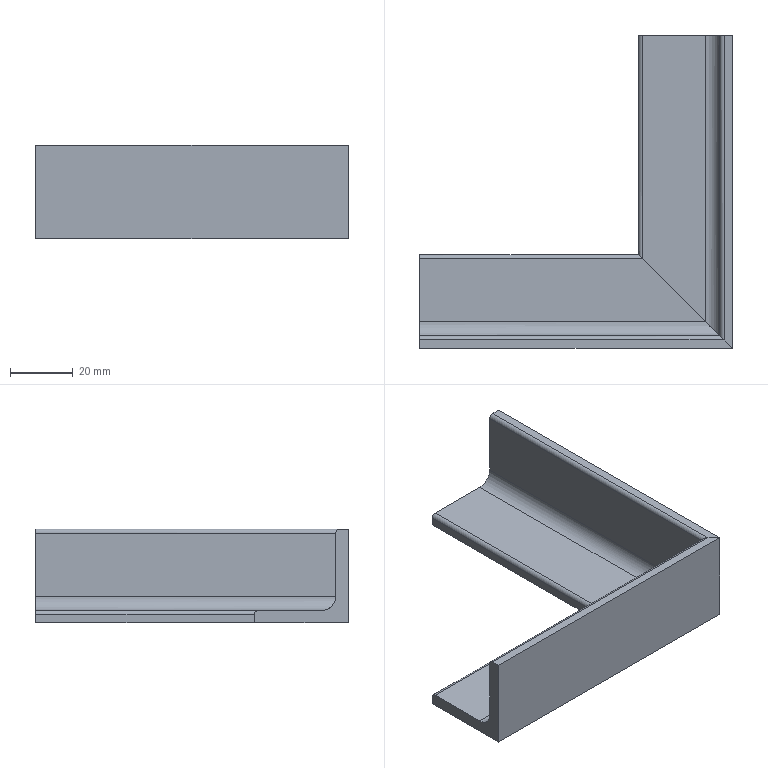Part | SolidWorks | features WeldMemberFeat 1, WeldmentFeature 1 | 2 solids | 22 faces | box 100 x 100 x 30 mm | volume 41483 mm3 | plane 16 | cylinder 6 | commonest cylinder face diameters 2.667 x4 9 x2
STEP:
#1=CARTESIAN_POINT('',(100.,0.,0.));
#2=VERTEX_POINT('',#1);
#3=CARTESIAN_POINT('',(70.,30.,0.));
#4=VERTEX_POINT('',#3);
#5=CARTESIAN_POINT('',(85.,15.,0.));
#6=DIRECTION('',(-0.7071,0.7071,0.));
#7=VECTOR('',#6,1000.);
#8=LINE('',#5,#7);
#9=EDGE_CURVE('',#2,#4,#8,.T.);
#10=ORIENTED_EDGE('',*,*,#9,.F.);
#11=CARTESIAN_POINT('',(0.,0.,0.));
#12=VERTEX_POINT('',#11);
#13=CARTESIAN_POINT('',(100.,0.,0.));
#14=DIRECTION('',(-1.,0.,0.));
#15=VECTOR('',#14,1000.);
#16=LINE('',#13,#15);
#17=EDGE_CURVE('',#2,#12,#16,.T.);
#18=ORIENTED_EDGE('',*,*,#17,.T.);
#19=CARTESIAN_POINT('',(0.,30.,0.));
#20=VERTEX_POINT('',#19);
#21=CARTESIAN_POINT('',(0.,30.,0.));
#22=DIRECTION('',(0.,1.,0.));
#23=VECTOR('',#22,1000.);
#24=LINE('',#21,#23);
#25=EDGE_CURVE('',#12,#20,#24,.T.);
#26=ORIENTED_EDGE('',*,*,#25,.T.);
#27=CARTESIAN_POINT('',(100.,30.,0.));
#28=DIRECTION('',(-1.,0.,0.));
#29=VECTOR('',#28,1000.);
#30=LINE('',#27,#29);
#31=EDGE_CURVE('',#4,#20,#30,.T.);
#32=ORIENTED_EDGE('',*,*,#31,.F.);
#33=EDGE_LOOP('',(#10,#18,#26,#32));
#34=FACE_OUTER_BOUND('',#33,.T.);
#35=CARTESIAN_POINT('',(100.,30.,0.));
#36=DIRECTION('',(0.,0.,1.));
#37=DIRECTION('',(1.,0.,0.));
#38=AXIS2_PLACEMENT_3D('',#35,#36,#37);
#39=PLANE('',#38);
#40=ADVANCED_FACE('',(#34),#39,.F.);
#41=CARTESIAN_POINT('',(70.,30.,2.667));
#42=VERTEX_POINT('',#41);
#43=CARTESIAN_POINT('',(70.,30.,0.));
#44=DIRECTION('',(0.,0.,1.));
#45=VECTOR('',#44,1000.);
#46=LINE('',#43,#45);
#47=EDGE_CURVE('',#4,#42,#46,.T.);
#48=ORIENTED_EDGE('',*,*,#47,.F.);
#49=ORIENTED_EDGE('',*,*,#31,.T.);
#50=CARTESIAN_POINT('',(0.,30.,2.667));
#51=VERTEX_POINT('',#50);
#52=CARTESIAN_POINT('',(0.,30.,0.));
#53=DIRECTION('',(0.,0.,1.));
#54=VECTOR('',#53,1000.);
#55=LINE('',#52,#54);
#56=EDGE_CURVE('',#20,#51,#55,.T.);
#57=ORIENTED_EDGE('',*,*,#56,.T.);
#58=CARTESIAN_POINT('',(100.,30.,2.667));
#59=DIRECTION('',(-1.,0.,0.));
#60=VECTOR('',#59,1000.);
#61=LINE('',#58,#60);
#62=EDGE_CURVE('',#42,#51,#61,.T.);
#63=ORIENTED_EDGE('',*,*,#62,.F.);
#64=EDGE_LOOP('',(#48,#49,#57,#63));
#65=FACE_OUTER_BOUND('',#64,.T.);
#66=CARTESIAN_POINT('',(100.,30.,0.));
#67=DIRECTION('',(0.,-1.,0.));
#68=DIRECTION('',(0.,0.,-1.));
#69=AXIS2_PLACEMENT_3D('',#66,#67,#68);
#70=PLANE('',#69);
#71=ADVANCED_FACE('',(#65),#70,.F.);
#72=CARTESIAN_POINT('',(71.333,28.667,4.));
#73=VERTEX_POINT('',#72);
#74=CARTESIAN_POINT('',(70.,30.,2.667));
#75=CARTESIAN_POINT('',(70.,30.,3.448));
#76=CARTESIAN_POINT('',(70.552,29.448,4.));
#77=CARTESIAN_POINT('',(71.333,28.667,4.));
#78=(BOUNDED_CURVE()B_SPLINE_CURVE(3,(#74,#75,#76,#77),.UNSPECIFIED.,.F.,.F.)B_SPLINE_CURVE_WITH_KNOTS((4,4),(0.,1.571),.UNSPECIFIED.)CURVE()GEOMETRIC_REPRESENTATION_ITEM()RATIONAL_B_SPLINE_CURVE((1.,0.8047,0.8047,1.))REPRESENTATION_ITEM(''));
#79=EDGE_CURVE('',#42,#73,#78,.T.);
#80=ORIENTED_EDGE('',*,*,#79,.F.);
#81=ORIENTED_EDGE('',*,*,#62,.T.);
#82=CARTESIAN_POINT('',(0.,28.667,4.));
#83=VERTEX_POINT('',#82);
#84=CARTESIAN_POINT('',(0.,28.667,2.667));
#85=DIRECTION('',(1.,0.,0.));
#86=DIRECTION('',(0.,0.,-1.));
#87=AXIS2_PLACEMENT_3D('',#84,#85,#86);
#88=CIRCLE('',#87,1.333);
#89=EDGE_CURVE('',#51,#83,#88,.T.);
#90=ORIENTED_EDGE('',*,*,#89,.T.);
#91=CARTESIAN_POINT('',(100.,28.667,4.));
#92=DIRECTION('',(-1.,0.,0.));
#93=VECTOR('',#92,1000.);
#94=LINE('',#91,#93);
#95=EDGE_CURVE('',#73,#83,#94,.T.);
#96=ORIENTED_EDGE('',*,*,#95,.F.);
#97=EDGE_LOOP('',(#80,#81,#90,#96));
#98=FACE_OUTER_BOUND('',#97,.T.);
#99=CARTESIAN_POINT('',(100.,28.667,2.667));
#100=DIRECTION('',(-1.,0.,0.));
#101=DIRECTION('',(0.,0.,1.));
#102=AXIS2_PLACEMENT_3D('',#99,#100,#101);
#103=CYLINDRICAL_SURFACE('',#102,1.333);
#104=ADVANCED_FACE('',(#98),#103,.T.);
#105=CARTESIAN_POINT('',(91.5,8.5,4.));
#106=VERTEX_POINT('',#105);
#107=CARTESIAN_POINT('',(95.75,4.25,4.));
#108=DIRECTION('',(0.7071,-0.7071,0.));
#109=VECTOR('',#108,1000.);
#110=LINE('',#107,#109);
#111=EDGE_CURVE('',#73,#106,#110,.T.);
#112=ORIENTED_EDGE('',*,*,#111,.F.);
#113=ORIENTED_EDGE('',*,*,#95,.T.);
#114=CARTESIAN_POINT('',(0.,8.5,4.));
#115=VERTEX_POINT('',#114);
#116=CARTESIAN_POINT('',(0.,8.5,4.));
#117=DIRECTION('',(0.,-1.,0.));
#118=VECTOR('',#117,1000.);
#119=LINE('',#116,#118);
#120=EDGE_CURVE('',#83,#115,#119,.T.);
#121=ORIENTED_EDGE('',*,*,#120,.T.);
#122=CARTESIAN_POINT('',(100.,8.5,4.));
#123=DIRECTION('',(-1.,0.,0.));
#124=VECTOR('',#123,1000.);
#125=LINE('',#122,#124);
#126=EDGE_CURVE('',#106,#115,#125,.T.);
#127=ORIENTED_EDGE('',*,*,#126,.F.);
#128=EDGE_LOOP('',(#112,#113,#121,#127));
#129=FACE_OUTER_BOUND('',#128,.T.);
#130=CARTESIAN_POINT('',(100.,8.5,4.));
#131=DIRECTION('',(0.,0.,-1.));
#132=DIRECTION('',(0.,1.,0.));
#133=AXIS2_PLACEMENT_3D('',#130,#131,#132);
#134=PLANE('',#133);
#135=ADVANCED_FACE('',(#129),#134,.F.);
#136=CARTESIAN_POINT('',(96.,4.,8.5));
#137=VERTEX_POINT('',#136);
#138=CARTESIAN_POINT('',(91.5,8.5,4.));
#139=CARTESIAN_POINT('',(94.136,5.864,4.));
#140=CARTESIAN_POINT('',(96.,4.,5.864));
#141=CARTESIAN_POINT('',(96.,4.,8.5));
#142=(BOUNDED_CURVE()B_SPLINE_CURVE(3,(#138,#139,#140,#141),.UNSPECIFIED.,.F.,.F.)B_SPLINE_CURVE_WITH_KNOTS((4,4),(1.571,3.142),.UNSPECIFIED.)CURVE()GEOMETRIC_REPRESENTATION_ITEM()RATIONAL_B_SPLINE_CURVE((1.,0.8047,0.8047,1.))REPRESENTATION_ITEM(''));
#143=EDGE_CURVE('',#106,#137,#142,.T.);
#144=ORIENTED_EDGE('',*,*,#143,.F.);
#145=ORIENTED_EDGE('',*,*,#126,.T.);
#146=CARTESIAN_POINT('',(0.,4.,8.5));
#147=VERTEX_POINT('',#146);
#148=CARTESIAN_POINT('',(0.,8.5,8.5));
#149=DIRECTION('',(-1.,0.,0.));
#150=DIRECTION('',(0.,0.,1.));
#151=AXIS2_PLACEMENT_3D('',#148,#149,#150);
#152=CIRCLE('',#151,4.5);
#153=EDGE_CURVE('',#115,#147,#152,.T.);
#154=ORIENTED_EDGE('',*,*,#153,.T.);
#155=CARTESIAN_POINT('',(100.,4.,8.5));
#156=DIRECTION('',(-1.,0.,0.));
#157=VECTOR('',#156,1000.);
#158=LINE('',#155,#157);
#159=EDGE_CURVE('',#137,#147,#158,.T.);
#160=ORIENTED_EDGE('',*,*,#159,.F.);
#161=EDGE_LOOP('',(#144,#145,#154,#160));
#162=FACE_OUTER_BOUND('',#161,.T.);
#163=CARTESIAN_POINT('',(100.,8.5,8.5));
#164=DIRECTION('',(-1.,0.,0.));
#165=DIRECTION('',(0.,0.,1.));
#166=AXIS2_PLACEMENT_3D('',#163,#164,#165);
#167=CYLINDRICAL_SURFACE('',#166,4.5);
#168=ADVANCED_FACE('',(#162),#167,.F.);
#169=CARTESIAN_POINT('',(96.,4.,28.667));
#170=VERTEX_POINT('',#169);
#171=CARTESIAN_POINT('',(96.,4.,28.667));
#172=DIRECTION('',(0.,0.,1.));
#173=VECTOR('',#172,1000.);
#174=LINE('',#171,#173);
#175=EDGE_CURVE('',#137,#170,#174,.T.);
#176=ORIENTED_EDGE('',*,*,#175,.F.);
#177=ORIENTED_EDGE('',*,*,#159,.T.);
#178=CARTESIAN_POINT('',(0.,4.,28.667));
#179=VERTEX_POINT('',#178);
#180=CARTESIAN_POINT('',(0.,4.,28.667));
#181=DIRECTION('',(0.,0.,1.));
#182=VECTOR('',#181,1000.);
#183=LINE('',#180,#182);
#184=EDGE_CURVE('',#147,#179,#183,.T.);
#185=ORIENTED_EDGE('',*,*,#184,.T.);
#186=CARTESIAN_POINT('',(100.,4.,28.667));
#187=DIRECTION('',(-1.,0.,0.));
#188=VECTOR('',#187,1000.);
#189=LINE('',#186,#188);
#190=EDGE_CURVE('',#170,#179,#189,.T.);
#191=ORIENTED_EDGE('',*,*,#190,.F.);
#192=EDGE_LOOP('',(#176,#177,#185,#191));
#193=FACE_OUTER_BOUND('',#192,.T.);
#194=CARTESIAN_POINT('',(100.,4.,28.667));
#195=DIRECTION('',(0.,-1.,0.));
#196=DIRECTION('',(0.,0.,-1.));
#197=AXIS2_PLACEMENT_3D('',#194,#195,#196);
#198=PLANE('',#197);
#199=ADVANCED_FACE('',(#193),#198,.F.);
#200=CARTESIAN_POINT('',(97.333,2.667,30.));
#201=VERTEX_POINT('',#200);
#202=CARTESIAN_POINT('',(96.,4.,28.667));
#203=CARTESIAN_POINT('',(96.,4.,29.448));
#204=CARTESIAN_POINT('',(96.552,3.448,30.));
#205=CARTESIAN_POINT('',(97.333,2.667,30.));
#206=(BOUNDED_CURVE()B_SPLINE_CURVE(3,(#202,#203,#204,#205),.UNSPECIFIED.,.F.,.F.)B_SPLINE_CURVE_WITH_KNOTS((4,4),(0.,1.571),.UNSPECIFIED.)CURVE()GEOMETRIC_REPRESENTATION_ITEM()RATIONAL_B_SPLINE_CURVE((1.,0.8047,0.8047,1.))REPRESENTATION_ITEM(''));
#207=EDGE_CURVE('',#170,#201,#206,.T.);
#208=ORIENTED_EDGE('',*,*,#207,.F.);
#209=ORIENTED_EDGE('',*,*,#190,.T.);
#210=CARTESIAN_POINT('',(0.,2.667,30.));
#211=VERTEX_POINT('',#210);
#212=CARTESIAN_POINT('',(0.,2.667,28.667));
#213=DIRECTION('',(1.,0.,0.));
#214=DIRECTION('',(0.,0.,1.));
#215=AXIS2_PLACEMENT_3D('',#212,#213,#214);
#216=CIRCLE('',#215,1.333);
#217=EDGE_CURVE('',#179,#211,#216,.T.);
#218=ORIENTED_EDGE('',*,*,#217,.T.);
#219=CARTESIAN_POINT('',(100.,2.667,30.));
#220=DIRECTION('',(-1.,0.,0.));
#221=VECTOR('',#220,1000.);
#222=LINE('',#219,#221);
#223=EDGE_CURVE('',#201,#211,#222,.T.);
#224=ORIENTED_EDGE('',*,*,#223,.F.);
#225=EDGE_LOOP('',(#208,#209,#218,#224));
#226=FACE_OUTER_BOUND('',#225,.T.);
#227=CARTESIAN_POINT('',(100.,2.667,28.667));
#228=DIRECTION('',(-1.,0.,0.));
#229=DIRECTION('',(0.,0.,1.));
#230=AXIS2_PLACEMENT_3D('',#227,#228,#229);
#231=CYLINDRICAL_SURFACE('',#230,1.333);
#232=ADVANCED_FACE('',(#226),#231,.T.);
#233=CARTESIAN_POINT('',(100.,0.,30.));
#234=VERTEX_POINT('',#233);
#235=CARTESIAN_POINT('',(100.,0.,30.));
#236=DIRECTION('',(0.7071,-0.7071,0.));
#237=VECTOR('',#236,1000.);
#238=LINE('',#235,#237);
#239=EDGE_CURVE('',#201,#234,#238,.T.);
#240=ORIENTED_EDGE('',*,*,#239,.F.);
#241=ORIENTED_EDGE('',*,*,#223,.T.);
#242=CARTESIAN_POINT('',(0.,0.,30.));
#243=VERTEX_POINT('',#242);
#244=CARTESIAN_POINT('',(0.,0.,30.));
#245=DIRECTION('',(0.,-1.,0.));
#246=VECTOR('',#245,1000.);
#247=LINE('',#244,#246);
#248=EDGE_CURVE('',#211,#243,#247,.T.);
#249=ORIENTED_EDGE('',*,*,#248,.T.);
#250=CARTESIAN_POINT('',(100.,0.,30.));
#251=DIRECTION('',(-1.,0.,0.));
#252=VECTOR('',#251,1000.);
#253=LINE('',#250,#252);
#254=EDGE_CURVE('',#234,#243,#253,.T.);
#255=ORIENTED_EDGE('',*,*,#254,.F.);
#256=EDGE_LOOP('',(#240,#241,#249,#255));
#257=FACE_OUTER_BOUND('',#256,.T.);
#258=CARTESIAN_POINT('',(100.,0.,30.));
#259=DIRECTION('',(0.,0.,-1.));
#260=DIRECTION('',(-1.,0.,0.));
#261=AXIS2_PLACEMENT_3D('',#258,#259,#260);
#262=PLANE('',#261);
#263=ADVANCED_FACE('',(#257),#262,.F.);
#264=CARTESIAN_POINT('',(100.,0.,0.));
#265=DIRECTION('',(0.,0.,-1.));
#266=VECTOR('',#265,1000.);
#267=LINE('',#264,#266);
#268=EDGE_CURVE('',#234,#2,#267,.T.);
#269=ORIENTED_EDGE('',*,*,#268,.F.);
#270=ORIENTED_EDGE('',*,*,#254,.T.);
#271=CARTESIAN_POINT('',(0.,0.,0.));
#272=DIRECTION('',(0.,0.,-1.));
#273=VECTOR('',#272,1000.);
#274=LINE('',#271,#273);
#275=EDGE_CURVE('',#243,#12,#274,.T.);
#276=ORIENTED_EDGE('',*,*,#275,.T.);
#277=ORIENTED_EDGE('',*,*,#17,.F.);
#278=EDGE_LOOP('',(#269,#270,#276,#277));
#279=FACE_OUTER_BOUND('',#278,.T.);
#280=CARTESIAN_POINT('',(100.,0.,0.));
#281=DIRECTION('',(0.,1.,0.));
#282=DIRECTION('',(0.,0.,1.));
#283=AXIS2_PLACEMENT_3D('',#280,#281,#282);
#284=PLANE('',#283);
#285=ADVANCED_FACE('',(#279),#284,.F.);
#286=ORIENTED_EDGE('',*,*,#25,.F.);
#287=ORIENTED_EDGE('',*,*,#275,.F.);
#288=ORIENTED_EDGE('',*,*,#248,.F.);
#289=ORIENTED_EDGE('',*,*,#217,.F.);
#290=ORIENTED_EDGE('',*,*,#184,.F.);
#291=ORIENTED_EDGE('',*,*,#153,.F.);
#292=ORIENTED_EDGE('',*,*,#120,.F.);
#293=ORIENTED_EDGE('',*,*,#89,.F.);
#294=ORIENTED_EDGE('',*,*,#56,.F.);
#295=EDGE_LOOP('',(#286,#287,#288,#289,#290,#291,#292,#293,#294));
#296=FACE_OUTER_BOUND('',#295,.T.);
#297=CARTESIAN_POINT('',(0.,2.667,28.667));
#298=DIRECTION('',(-1.,0.,0.));
#299=DIRECTION('',(0.,0.,1.));
#300=AXIS2_PLACEMENT_3D('',#297,#298,#299);
#301=PLANE('',#300);
#302=ADVANCED_FACE('',(#296),#301,.T.);
#303=ORIENTED_EDGE('',*,*,#268,.T.);
#304=ORIENTED_EDGE('',*,*,#9,.T.);
#305=ORIENTED_EDGE('',*,*,#47,.T.);
#306=ORIENTED_EDGE('',*,*,#79,.T.);
#307=ORIENTED_EDGE('',*,*,#111,.T.);
#308=ORIENTED_EDGE('',*,*,#143,.T.);
#309=ORIENTED_EDGE('',*,*,#175,.T.);
#310=ORIENTED_EDGE('',*,*,#207,.T.);
#311=ORIENTED_EDGE('',*,*,#239,.T.);
#312=EDGE_LOOP('',(#303,#304,#305,#306,#307,#308,#309,#310,#311));
#313=FACE_OUTER_BOUND('',#312,.T.);
#314=CARTESIAN_POINT('',(100.,0.,0.));
#315=DIRECTION('',(0.7071,0.7071,0.));
#316=DIRECTION('',(-0.7071,0.7071,0.));
#317=AXIS2_PLACEMENT_3D('',#314,#315,#316);
#318=PLANE('',#317);
#319=ADVANCED_FACE('',(#313),#318,.T.);
#320=CLOSED_SHELL('',(#40,#71,#104,#135,#168,#199,#232,#263,#285,#302,#319));
#321=MANIFOLD_SOLID_BREP('',#320);
#322=CARTESIAN_POINT('',(70.,30.,0.));
#323=VERTEX_POINT('',#322);
#324=CARTESIAN_POINT('',(100.,0.,0.));
#325=VERTEX_POINT('',#324);
#326=CARTESIAN_POINT('',(35.,65.,0.));
#327=DIRECTION('',(0.7071,-0.7071,0.));
#328=VECTOR('',#327,1000.);
#329=LINE('',#326,#328);
#330=EDGE_CURVE('',#323,#325,#329,.T.);
#331=ORIENTED_EDGE('',*,*,#330,.F.);
#332=CARTESIAN_POINT('',(70.,100.,0.));
#333=VERTEX_POINT('',#332);
#334=CARTESIAN_POINT('',(70.,100.,0.));
#335=DIRECTION('',(0.,-1.,0.));
#336=VECTOR('',#335,1000.);
#337=LINE('',#334,#336);
#338=EDGE_CURVE('',#333,#323,#337,.T.);
#339=ORIENTED_EDGE('',*,*,#338,.F.);
#340=CARTESIAN_POINT('',(100.,100.,0.));
#341=VERTEX_POINT('',#340);
#342=CARTESIAN_POINT('',(70.,100.,0.));
#343=DIRECTION('',(-1.,0.,0.));
#344=VECTOR('',#343,1000.);
#345=LINE('',#342,#344);
#346=EDGE_CURVE('',#341,#333,#345,.T.);
#347=ORIENTED_EDGE('',*,*,#346,.F.);
#348=CARTESIAN_POINT('',(100.,100.,0.));
#349=DIRECTION('',(0.,-1.,0.));
#350=VECTOR('',#349,1000.);
#351=LINE('',#348,#350);
#352=EDGE_CURVE('',#341,#325,#351,.T.);
#353=ORIENTED_EDGE('',*,*,#352,.T.);
#354=EDGE_LOOP('',(#331,#339,#347,#353));
#355=FACE_OUTER_BOUND('',#354,.T.);
#356=CARTESIAN_POINT('',(70.,100.,0.));
#357=DIRECTION('',(0.,0.,1.));
#358=DIRECTION('',(1.,0.,0.));
#359=AXIS2_PLACEMENT_3D('',#356,#357,#358);
#360=PLANE('',#359);
#361=ADVANCED_FACE('',(#355),#360,.F.);
#362=CARTESIAN_POINT('',(70.,30.,2.667));
#363=VERTEX_POINT('',#362);
#364=CARTESIAN_POINT('',(70.,30.,0.));
#365=DIRECTION('',(0.,0.,-1.));
#366=VECTOR('',#365,1000.);
#367=LINE('',#364,#366);
#368=EDGE_CURVE('',#363,#323,#367,.T.);
#369=ORIENTED_EDGE('',*,*,#368,.F.);
#370=CARTESIAN_POINT('',(70.,100.,2.667));
#371=VERTEX_POINT('',#370);
#372=CARTESIAN_POINT('',(70.,100.,2.667));
#373=DIRECTION('',(0.,-1.,0.));
#374=VECTOR('',#373,1000.);
#375=LINE('',#372,#374);
#376=EDGE_CURVE('',#371,#363,#375,.T.);
#377=ORIENTED_EDGE('',*,*,#376,.F.);
#378=CARTESIAN_POINT('',(70.,100.,0.));
#379=DIRECTION('',(0.,0.,1.));
#380=VECTOR('',#379,1000.);
#381=LINE('',#378,#380);
#382=EDGE_CURVE('',#333,#371,#381,.T.);
#383=ORIENTED_EDGE('',*,*,#382,.F.);
#384=ORIENTED_EDGE('',*,*,#338,.T.);
#385=EDGE_LOOP('',(#369,#377,#383,#384));
#386=FACE_OUTER_BOUND('',#385,.T.);
#387=CARTESIAN_POINT('',(70.,100.,0.));
#388=DIRECTION('',(1.,0.,0.));
#389=DIRECTION('',(0.,0.,-1.));
#390=AXIS2_PLACEMENT_3D('',#387,#388,#389);
#391=PLANE('',#390);
#392=ADVANCED_FACE('',(#386),#391,.F.);
#393=CARTESIAN_POINT('',(71.333,28.667,4.));
#394=VERTEX_POINT('',#393);
#395=CARTESIAN_POINT('',(71.333,28.667,4.));
#396=CARTESIAN_POINT('',(70.552,29.448,4.));
#397=CARTESIAN_POINT('',(70.,30.,3.448));
#398=CARTESIAN_POINT('',(70.,30.,2.667));
#399=(BOUNDED_CURVE()B_SPLINE_CURVE(3,(#395,#396,#397,#398),.UNSPECIFIED.,.F.,.F.)B_SPLINE_CURVE_WITH_KNOTS((4,4),(1.571,3.142),.UNSPECIFIED.)CURVE()GEOMETRIC_REPRESENTATION_ITEM()RATIONAL_B_SPLINE_CURVE((1.,0.8047,0.8047,1.))REPRESENTATION_ITEM(''));
#400=EDGE_CURVE('',#394,#363,#399,.T.);
#401=ORIENTED_EDGE('',*,*,#400,.F.);
#402=CARTESIAN_POINT('',(71.333,100.,4.));
#403=VERTEX_POINT('',#402);
#404=CARTESIAN_POINT('',(71.333,100.,4.));
#405=DIRECTION('',(0.,-1.,0.));
#406=VECTOR('',#405,1000.);
#407=LINE('',#404,#406);
#408=EDGE_CURVE('',#403,#394,#407,.T.);
#409=ORIENTED_EDGE('',*,*,#408,.F.);
#410=CARTESIAN_POINT('',(71.333,100.,2.667));
#411=DIRECTION('',(0.,1.,0.));
#412=DIRECTION('',(0.,0.,-1.));
#413=AXIS2_PLACEMENT_3D('',#410,#411,#412);
#414=CIRCLE('',#413,1.333);
#415=EDGE_CURVE('',#371,#403,#414,.T.);
#416=ORIENTED_EDGE('',*,*,#415,.F.);
#417=ORIENTED_EDGE('',*,*,#376,.T.);
#418=EDGE_LOOP('',(#401,#409,#416,#417));
#419=FACE_OUTER_BOUND('',#418,.T.);
#420=CARTESIAN_POINT('',(71.333,100.,2.667));
#421=DIRECTION('',(0.,-1.,0.));
#422=DIRECTION('',(0.,0.,-1.));
#423=AXIS2_PLACEMENT_3D('',#420,#421,#422);
#424=CYLINDRICAL_SURFACE('',#423,1.333);
#425=ADVANCED_FACE('',(#419),#424,.T.);
#426=CARTESIAN_POINT('',(91.5,8.5,4.));
#427=VERTEX_POINT('',#426);
#428=CARTESIAN_POINT('',(45.75,54.25,4.));
#429=DIRECTION('',(-0.7071,0.7071,0.));
#430=VECTOR('',#429,1000.);
#431=LINE('',#428,#430);
#432=EDGE_CURVE('',#427,#394,#431,.T.);
#433=ORIENTED_EDGE('',*,*,#432,.F.);
#434=CARTESIAN_POINT('',(91.5,100.,4.));
#435=VERTEX_POINT('',#434);
#436=CARTESIAN_POINT('',(91.5,100.,4.));
#437=DIRECTION('',(0.,-1.,0.));
#438=VECTOR('',#437,1000.);
#439=LINE('',#436,#438);
#440=EDGE_CURVE('',#435,#427,#439,.T.);
#441=ORIENTED_EDGE('',*,*,#440,.F.);
#442=CARTESIAN_POINT('',(91.5,100.,4.));
#443=DIRECTION('',(1.,0.,0.));
#444=VECTOR('',#443,1000.);
#445=LINE('',#442,#444);
#446=EDGE_CURVE('',#403,#435,#445,.T.);
#447=ORIENTED_EDGE('',*,*,#446,.F.);
#448=ORIENTED_EDGE('',*,*,#408,.T.);
#449=EDGE_LOOP('',(#433,#441,#447,#448));
#450=FACE_OUTER_BOUND('',#449,.T.);
#451=CARTESIAN_POINT('',(91.5,100.,4.));
#452=DIRECTION('',(0.,0.,-1.));
#453=DIRECTION('',(-1.,0.,0.));
#454=AXIS2_PLACEMENT_3D('',#451,#452,#453);
#455=PLANE('',#454);
#456=ADVANCED_FACE('',(#450),#455,.F.);
#457=CARTESIAN_POINT('',(96.,4.,8.5));
#458=VERTEX_POINT('',#457);
#459=CARTESIAN_POINT('',(96.,4.,8.5));
#460=CARTESIAN_POINT('',(96.,4.,5.864));
#461=CARTESIAN_POINT('',(94.136,5.864,4.));
#462=CARTESIAN_POINT('',(91.5,8.5,4.));
#463=(BOUNDED_CURVE()B_SPLINE_CURVE(3,(#459,#460,#461,#462),.UNSPECIFIED.,.F.,.F.)B_SPLINE_CURVE_WITH_KNOTS((4,4),(0.,1.571),.UNSPECIFIED.)CURVE()GEOMETRIC_REPRESENTATION_ITEM()RATIONAL_B_SPLINE_CURVE((1.,0.8047,0.8047,1.))REPRESENTATION_ITEM(''));
#464=EDGE_CURVE('',#458,#427,#463,.T.);
#465=ORIENTED_EDGE('',*,*,#464,.F.);
#466=CARTESIAN_POINT('',(96.,100.,8.5));
#467=VERTEX_POINT('',#466);
#468=CARTESIAN_POINT('',(96.,100.,8.5));
#469=DIRECTION('',(0.,-1.,0.));
#470=VECTOR('',#469,1000.);
#471=LINE('',#468,#470);
#472=EDGE_CURVE('',#467,#458,#471,.T.);
#473=ORIENTED_EDGE('',*,*,#472,.F.);
#474=CARTESIAN_POINT('',(91.5,100.,8.5));
#475=DIRECTION('',(0.,-1.,0.));
#476=DIRECTION('',(0.,0.,1.));
#477=AXIS2_PLACEMENT_3D('',#474,#475,#476);
#478=CIRCLE('',#477,4.5);
#479=EDGE_CURVE('',#435,#467,#478,.T.);
#480=ORIENTED_EDGE('',*,*,#479,.F.);
#481=ORIENTED_EDGE('',*,*,#440,.T.);
#482=EDGE_LOOP('',(#465,#473,#480,#481));
#483=FACE_OUTER_BOUND('',#482,.T.);
#484=CARTESIAN_POINT('',(91.5,100.,8.5));
#485=DIRECTION('',(0.,-1.,0.));
#486=DIRECTION('',(0.,0.,-1.));
#487=AXIS2_PLACEMENT_3D('',#484,#485,#486);
#488=CYLINDRICAL_SURFACE('',#487,4.5);
#489=ADVANCED_FACE('',(#483),#488,.F.);
#490=CARTESIAN_POINT('',(96.,4.,28.667));
#491=VERTEX_POINT('',#490);
#492=CARTESIAN_POINT('',(96.,4.,28.667));
#493=DIRECTION('',(0.,0.,-1.));
#494=VECTOR('',#493,1000.);
#495=LINE('',#492,#494);
#496=EDGE_CURVE('',#491,#458,#495,.T.);
#497=ORIENTED_EDGE('',*,*,#496,.F.);
#498=CARTESIAN_POINT('',(96.,100.,28.667));
#499=VERTEX_POINT('',#498);
#500=CARTESIAN_POINT('',(96.,100.,28.667));
#501=DIRECTION('',(0.,-1.,0.));
#502=VECTOR('',#501,1000.);
#503=LINE('',#500,#502);
#504=EDGE_CURVE('',#499,#491,#503,.T.);
#505=ORIENTED_EDGE('',*,*,#504,.F.);
#506=CARTESIAN_POINT('',(96.,100.,28.667));
#507=DIRECTION('',(0.,0.,1.));
#508=VECTOR('',#507,1000.);
#509=LINE('',#506,#508);
#510=EDGE_CURVE('',#467,#499,#509,.T.);
#511=ORIENTED_EDGE('',*,*,#510,.F.);
#512=ORIENTED_EDGE('',*,*,#472,.T.);
#513=EDGE_LOOP('',(#497,#505,#511,#512));
#514=FACE_OUTER_BOUND('',#513,.T.);
#515=CARTESIAN_POINT('',(96.,100.,28.667));
#516=DIRECTION('',(1.,0.,0.));
#517=DIRECTION('',(0.,0.,-1.));
#518=AXIS2_PLACEMENT_3D('',#515,#516,#517);
#519=PLANE('',#518);
#520=ADVANCED_FACE('',(#514),#519,.F.);
#521=CARTESIAN_POINT('',(97.333,2.667,30.));
#522=VERTEX_POINT('',#521);
#523=CARTESIAN_POINT('',(97.333,2.667,30.));
#524=CARTESIAN_POINT('',(96.552,3.448,30.));
#525=CARTESIAN_POINT('',(96.,4.,29.448));
#526=CARTESIAN_POINT('',(96.,4.,28.667));
#527=(BOUNDED_CURVE()B_SPLINE_CURVE(3,(#523,#524,#525,#526),.UNSPECIFIED.,.F.,.F.)B_SPLINE_CURVE_WITH_KNOTS((4,4),(1.571,3.142),.UNSPECIFIED.)CURVE()GEOMETRIC_REPRESENTATION_ITEM()RATIONAL_B_SPLINE_CURVE((1.,0.8047,0.8047,1.))REPRESENTATION_ITEM(''));
#528=EDGE_CURVE('',#522,#491,#527,.T.);
#529=ORIENTED_EDGE('',*,*,#528,.F.);
#530=CARTESIAN_POINT('',(97.333,100.,30.));
#531=VERTEX_POINT('',#530);
#532=CARTESIAN_POINT('',(97.333,100.,30.));
#533=DIRECTION('',(0.,-1.,0.));
#534=VECTOR('',#533,1000.);
#535=LINE('',#532,#534);
#536=EDGE_CURVE('',#531,#522,#535,.T.);
#537=ORIENTED_EDGE('',*,*,#536,.F.);
#538=CARTESIAN_POINT('',(97.333,100.,28.667));
#539=DIRECTION('',(0.,1.,0.));
#540=DIRECTION('',(0.,0.,1.));
#541=AXIS2_PLACEMENT_3D('',#538,#539,#540);
#542=CIRCLE('',#541,1.333);
#543=EDGE_CURVE('',#499,#531,#542,.T.);
#544=ORIENTED_EDGE('',*,*,#543,.F.);
#545=ORIENTED_EDGE('',*,*,#504,.T.);
#546=EDGE_LOOP('',(#529,#537,#544,#545));
#547=FACE_OUTER_BOUND('',#546,.T.);
#548=CARTESIAN_POINT('',(97.333,100.,28.667));
#549=DIRECTION('',(0.,-1.,0.));
#550=DIRECTION('',(0.,0.,-1.));
#551=AXIS2_PLACEMENT_3D('',#548,#549,#550);
#552=CYLINDRICAL_SURFACE('',#551,1.333);
#553=ADVANCED_FACE('',(#547),#552,.T.);
#554=CARTESIAN_POINT('',(100.,0.,30.));
#555=VERTEX_POINT('',#554);
#556=CARTESIAN_POINT('',(50.,50.,30.));
#557=DIRECTION('',(-0.7071,0.7071,0.));
#558=VECTOR('',#557,1000.);
#559=LINE('',#556,#558);
#560=EDGE_CURVE('',#555,#522,#559,.T.);
#561=ORIENTED_EDGE('',*,*,#560,.F.);
#562=CARTESIAN_POINT('',(100.,100.,30.));
#563=VERTEX_POINT('',#562);
#564=CARTESIAN_POINT('',(100.,100.,30.));
#565=DIRECTION('',(0.,-1.,0.));
#566=VECTOR('',#565,1000.);
#567=LINE('',#564,#566);
#568=EDGE_CURVE('',#563,#555,#567,.T.);
#569=ORIENTED_EDGE('',*,*,#568,.F.);
#570=CARTESIAN_POINT('',(100.,100.,30.));
#571=DIRECTION('',(1.,0.,0.));
#572=VECTOR('',#571,1000.);
#573=LINE('',#570,#572);
#574=EDGE_CURVE('',#531,#563,#573,.T.);
#575=ORIENTED_EDGE('',*,*,#574,.F.);
#576=ORIENTED_EDGE('',*,*,#536,.T.);
#577=EDGE_LOOP('',(#561,#569,#575,#576));
#578=FACE_OUTER_BOUND('',#577,.T.);
#579=CARTESIAN_POINT('',(100.,100.,30.));
#580=DIRECTION('',(0.,0.,-1.));
#581=DIRECTION('',(-1.,0.,0.));
#582=AXIS2_PLACEMENT_3D('',#579,#580,#581);
#583=PLANE('',#582);
#584=ADVANCED_FACE('',(#578),#583,.F.);
#585=CARTESIAN_POINT('',(100.,0.,0.));
#586=DIRECTION('',(0.,0.,1.));
#587=VECTOR('',#586,1000.);
#588=LINE('',#585,#587);
#589=EDGE_CURVE('',#325,#555,#588,.T.);
#590=ORIENTED_EDGE('',*,*,#589,.F.);
#591=ORIENTED_EDGE('',*,*,#352,.F.);
#592=CARTESIAN_POINT('',(100.,100.,0.));
#593=DIRECTION('',(0.,0.,-1.));
#594=VECTOR('',#593,1000.);
#595=LINE('',#592,#594);
#596=EDGE_CURVE('',#563,#341,#595,.T.);
#597=ORIENTED_EDGE('',*,*,#596,.F.);
#598=ORIENTED_EDGE('',*,*,#568,.T.);
#599=EDGE_LOOP('',(#590,#591,#597,#598));
#600=FACE_OUTER_BOUND('',#599,.T.);
#601=CARTESIAN_POINT('',(100.,100.,0.));
#602=DIRECTION('',(-1.,0.,0.));
#603=DIRECTION('',(0.,0.,1.));
#604=AXIS2_PLACEMENT_3D('',#601,#602,#603);
#605=PLANE('',#604);
#606=ADVANCED_FACE('',(#600),#605,.F.);
#607=ORIENTED_EDGE('',*,*,#346,.T.);
#608=ORIENTED_EDGE('',*,*,#382,.T.);
#609=ORIENTED_EDGE('',*,*,#415,.T.);
#610=ORIENTED_EDGE('',*,*,#446,.T.);
#611=ORIENTED_EDGE('',*,*,#479,.T.);
#612=ORIENTED_EDGE('',*,*,#510,.T.);
#613=ORIENTED_EDGE('',*,*,#543,.T.);
#614=ORIENTED_EDGE('',*,*,#574,.T.);
#615=ORIENTED_EDGE('',*,*,#596,.T.);
#616=EDGE_LOOP('',(#607,#608,#609,#610,#611,#612,#613,#614,#615));
#617=FACE_OUTER_BOUND('',#616,.T.);
#618=CARTESIAN_POINT('',(97.333,100.,28.667));
#619=DIRECTION('',(0.,-1.,0.));
#620=DIRECTION('',(0.,0.,1.));
#621=AXIS2_PLACEMENT_3D('',#618,#619,#620);
#622=PLANE('',#621);
#623=ADVANCED_FACE('',(#617),#622,.F.);
#624=ORIENTED_EDGE('',*,*,#368,.T.);
#625=ORIENTED_EDGE('',*,*,#330,.T.);
#626=ORIENTED_EDGE('',*,*,#589,.T.);
#627=ORIENTED_EDGE('',*,*,#560,.T.);
#628=ORIENTED_EDGE('',*,*,#528,.T.);
#629=ORIENTED_EDGE('',*,*,#496,.T.);
#630=ORIENTED_EDGE('',*,*,#464,.T.);
#631=ORIENTED_EDGE('',*,*,#432,.T.);
#632=ORIENTED_EDGE('',*,*,#400,.T.);
#633=EDGE_LOOP('',(#624,#625,#626,#627,#628,#629,#630,#631,#632));
#634=FACE_OUTER_BOUND('',#633,.T.);
#635=CARTESIAN_POINT('',(100.,0.,0.));
#636=DIRECTION('',(-0.7071,-0.7071,0.));
#637=DIRECTION('',(0.7071,-0.7071,0.));
#638=AXIS2_PLACEMENT_3D('',#635,#636,#637);
#639=PLANE('',#638);
#640=ADVANCED_FACE('',(#634),#639,.T.);
#641=CLOSED_SHELL('',(#361,#392,#425,#456,#489,#520,#553,#584,#606,#623,#640));
#642=MANIFOLD_SOLID_BREP('',#641);
#643=CARTESIAN_POINT('',(0.,0.,0.));
#644=DIRECTION('',(0.,0.,1.));
#645=DIRECTION('',(1.,0.,0.));
#646=AXIS2_PLACEMENT_3D('',#643,#644,#645);
#647=(LENGTH_UNIT()NAMED_UNIT(*)SI_UNIT(.MILLI.,.METRE.));
#648=UNCERTAINTY_MEASURE_WITH_UNIT(LENGTH_MEASURE(0.00001),#647,'','');
#649=(NAMED_UNIT(*)PLANE_ANGLE_UNIT()SI_UNIT($,.RADIAN.));
#650=(NAMED_UNIT(*)SI_UNIT($,.STERADIAN.)SOLID_ANGLE_UNIT());
#651=(GEOMETRIC_REPRESENTATION_CONTEXT(3)GLOBAL_UNCERTAINTY_ASSIGNED_CONTEXT((#648))GLOBAL_UNIT_ASSIGNED_CONTEXT((#647,#649,#650))REPRESENTATION_CONTEXT('',''));
#652=ADVANCED_BREP_SHAPE_REPRESENTATION('',(#321,#642,#646),#651);